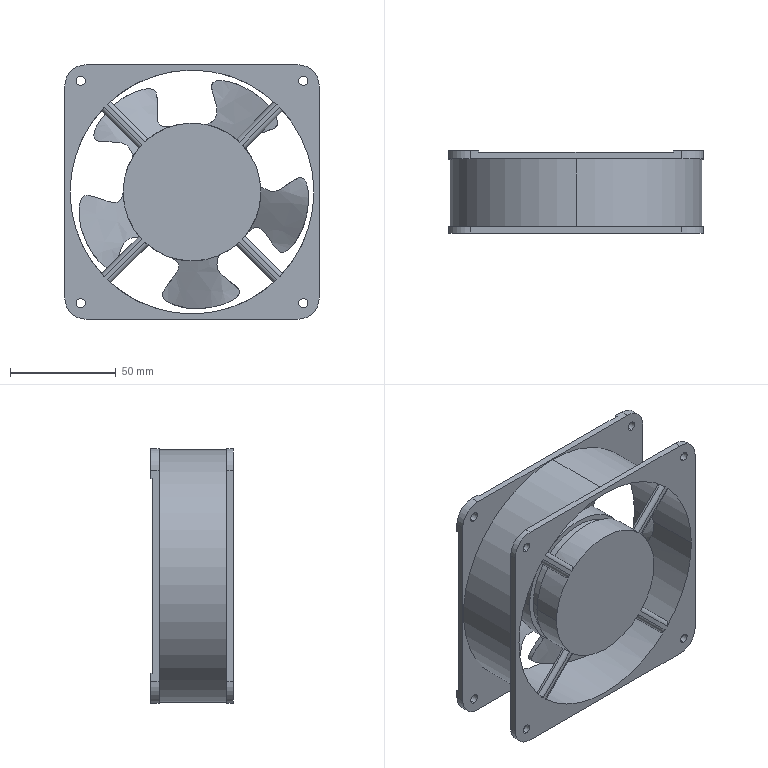Part | STEP file | 1 solid | 101 faces | box 120 x 38.9 x 120 mm | volume 179083 mm3 | cylinder 42 | plane 39 | spline 20 | commonest cylinder face diameters 4.4 x16 4 x8 20 x8 65 x4 60 x2 115 x2